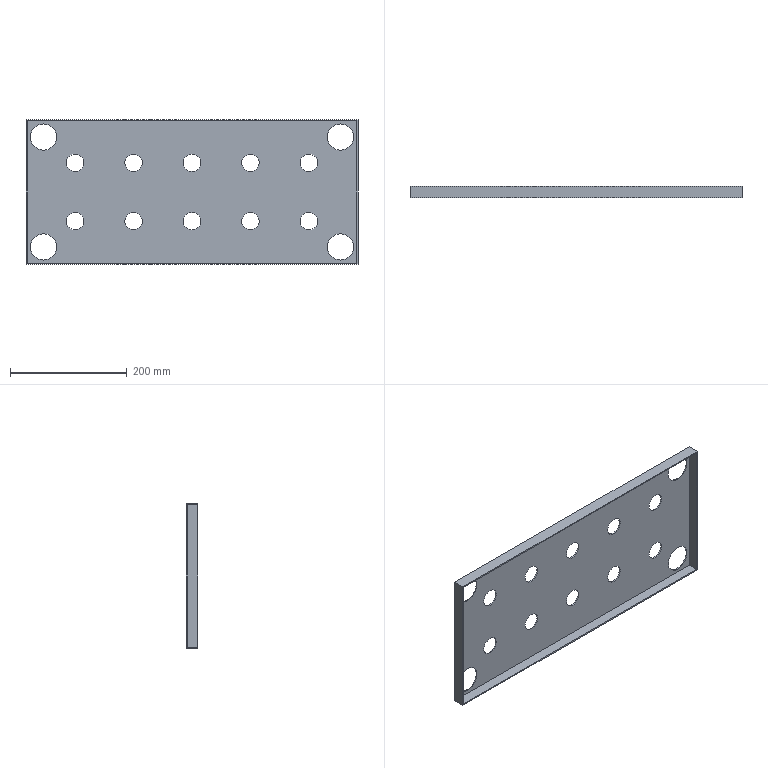Part | NX | 1 solid | 25 faces | box 568 x 20 x 248 mm | volume 313331 mm3 | cylinder 14 | plane 11 | commonest cylinder face diameters 30 x10 45 x4
STEP:
#1=CARTESIAN_POINT('',(-284.,0.,-124.));
#2=VERTEX_POINT('',#1);
#3=CARTESIAN_POINT('',(284.,0.,-124.));
#4=VERTEX_POINT('',#3);
#5=CARTESIAN_POINT('',(284.,0.,-124.));
#6=DIRECTION('',(1.,0.,0.));
#7=VECTOR('',#6,1000.);
#8=LINE('',#5,#7);
#9=EDGE_CURVE('',#2,#4,#8,.T.);
#10=ORIENTED_EDGE('',*,*,#9,.F.);
#11=CARTESIAN_POINT('',(-284.,20.,-124.));
#12=VERTEX_POINT('',#11);
#13=CARTESIAN_POINT('',(-284.,20.,-124.));
#14=DIRECTION('',(0.,-1.,0.));
#15=VECTOR('',#14,1000.);
#16=LINE('',#13,#15);
#17=EDGE_CURVE('',#12,#2,#16,.T.);
#18=ORIENTED_EDGE('',*,*,#17,.F.);
#19=CARTESIAN_POINT('',(284.,20.,-124.));
#20=VERTEX_POINT('',#19);
#21=CARTESIAN_POINT('',(284.,20.,-124.));
#22=DIRECTION('',(1.,0.,0.));
#23=VECTOR('',#22,1000.);
#24=LINE('',#21,#23);
#25=EDGE_CURVE('',#12,#20,#24,.T.);
#26=ORIENTED_EDGE('',*,*,#25,.T.);
#27=CARTESIAN_POINT('',(284.,20.,-124.));
#28=DIRECTION('',(0.,-1.,0.));
#29=VECTOR('',#28,1000.);
#30=LINE('',#27,#29);
#31=EDGE_CURVE('',#20,#4,#30,.T.);
#32=ORIENTED_EDGE('',*,*,#31,.T.);
#33=EDGE_LOOP('',(#10,#18,#26,#32));
#34=FACE_BOUND('',#33,.T.);
#35=CARTESIAN_POINT('',(284.,20.,-124.));
#36=DIRECTION('',(0.,0.,-1.));
#37=DIRECTION('',(-1.,0.,0.));
#38=AXIS2_PLACEMENT_3D('',#35,#36,#37);
#39=PLANE('',#38);
#40=ADVANCED_FACE('',(#34),#39,.T.);
#41=CARTESIAN_POINT('',(-284.,0.,124.));
#42=VERTEX_POINT('',#41);
#43=CARTESIAN_POINT('',(-284.,0.,124.));
#44=DIRECTION('',(0.,0.,-1.));
#45=VECTOR('',#44,1000.);
#46=LINE('',#43,#45);
#47=EDGE_CURVE('',#42,#2,#46,.T.);
#48=ORIENTED_EDGE('',*,*,#47,.F.);
#49=CARTESIAN_POINT('',(-284.,20.,124.));
#50=VERTEX_POINT('',#49);
#51=CARTESIAN_POINT('',(-284.,20.,124.));
#52=DIRECTION('',(0.,-1.,0.));
#53=VECTOR('',#52,1000.);
#54=LINE('',#51,#53);
#55=EDGE_CURVE('',#50,#42,#54,.T.);
#56=ORIENTED_EDGE('',*,*,#55,.F.);
#57=CARTESIAN_POINT('',(-284.,20.,124.));
#58=DIRECTION('',(0.,0.,-1.));
#59=VECTOR('',#58,1000.);
#60=LINE('',#57,#59);
#61=EDGE_CURVE('',#50,#12,#60,.T.);
#62=ORIENTED_EDGE('',*,*,#61,.T.);
#63=ORIENTED_EDGE('',*,*,#17,.T.);
#64=EDGE_LOOP('',(#48,#56,#62,#63));
#65=FACE_BOUND('',#64,.T.);
#66=CARTESIAN_POINT('',(-284.,20.,124.));
#67=DIRECTION('',(-1.,0.,0.));
#68=DIRECTION('',(0.,0.,1.));
#69=AXIS2_PLACEMENT_3D('',#66,#67,#68);
#70=PLANE('',#69);
#71=ADVANCED_FACE('',(#65),#70,.T.);
#72=CARTESIAN_POINT('',(284.,0.,124.));
#73=VERTEX_POINT('',#72);
#74=CARTESIAN_POINT('',(284.,0.,124.));
#75=DIRECTION('',(-1.,0.,0.));
#76=VECTOR('',#75,1000.);
#77=LINE('',#74,#76);
#78=EDGE_CURVE('',#73,#42,#77,.T.);
#79=ORIENTED_EDGE('',*,*,#78,.F.);
#80=CARTESIAN_POINT('',(284.,20.,124.));
#81=VERTEX_POINT('',#80);
#82=CARTESIAN_POINT('',(284.,20.,124.));
#83=DIRECTION('',(0.,-1.,0.));
#84=VECTOR('',#83,1000.);
#85=LINE('',#82,#84);
#86=EDGE_CURVE('',#81,#73,#85,.T.);
#87=ORIENTED_EDGE('',*,*,#86,.F.);
#88=CARTESIAN_POINT('',(284.,20.,124.));
#89=DIRECTION('',(-1.,0.,0.));
#90=VECTOR('',#89,1000.);
#91=LINE('',#88,#90);
#92=EDGE_CURVE('',#81,#50,#91,.T.);
#93=ORIENTED_EDGE('',*,*,#92,.T.);
#94=ORIENTED_EDGE('',*,*,#55,.T.);
#95=EDGE_LOOP('',(#79,#87,#93,#94));
#96=FACE_BOUND('',#95,.T.);
#97=CARTESIAN_POINT('',(284.,20.,124.));
#98=DIRECTION('',(0.,0.,1.));
#99=DIRECTION('',(1.,0.,0.));
#100=AXIS2_PLACEMENT_3D('',#97,#98,#99);
#101=PLANE('',#100);
#102=ADVANCED_FACE('',(#96),#101,.T.);
#103=CARTESIAN_POINT('',(284.,0.,124.));
#104=DIRECTION('',(0.,0.,1.));
#105=VECTOR('',#104,1000.);
#106=LINE('',#103,#105);
#107=EDGE_CURVE('',#4,#73,#106,.T.);
#108=ORIENTED_EDGE('',*,*,#107,.F.);
#109=ORIENTED_EDGE('',*,*,#31,.F.);
#110=CARTESIAN_POINT('',(284.,20.,124.));
#111=DIRECTION('',(0.,0.,1.));
#112=VECTOR('',#111,1000.);
#113=LINE('',#110,#112);
#114=EDGE_CURVE('',#20,#81,#113,.T.);
#115=ORIENTED_EDGE('',*,*,#114,.T.);
#116=ORIENTED_EDGE('',*,*,#86,.T.);
#117=EDGE_LOOP('',(#108,#109,#115,#116));
#118=FACE_BOUND('',#117,.T.);
#119=CARTESIAN_POINT('',(284.,20.,124.));
#120=DIRECTION('',(1.,0.,0.));
#121=DIRECTION('',(0.,0.,-1.));
#122=AXIS2_PLACEMENT_3D('',#119,#120,#121);
#123=PLANE('',#122);
#124=ADVANCED_FACE('',(#118),#123,.T.);
#125=CARTESIAN_POINT('',(-100.,20.,65.));
#126=VERTEX_POINT('',#125);
#127=CARTESIAN_POINT('',(-100.,20.,50.));
#128=DIRECTION('',(0.,1.,0.));
#129=DIRECTION('',(0.,0.,1.));
#130=AXIS2_PLACEMENT_3D('',#127,#128,#129);
#131=CIRCLE('',#130,15.);
#132=EDGE_CURVE('',#126,#126,#131,.T.);
#133=ORIENTED_EDGE('',*,*,#132,.F.);
#134=EDGE_LOOP('',(#133));
#135=FACE_BOUND('',#134,.T.);
#136=CARTESIAN_POINT('',(-200.,20.,65.));
#137=VERTEX_POINT('',#136);
#138=CARTESIAN_POINT('',(-200.,20.,50.));
#139=DIRECTION('',(0.,1.,0.));
#140=DIRECTION('',(0.,0.,1.));
#141=AXIS2_PLACEMENT_3D('',#138,#139,#140);
#142=CIRCLE('',#141,15.);
#143=EDGE_CURVE('',#137,#137,#142,.T.);
#144=ORIENTED_EDGE('',*,*,#143,.F.);
#145=EDGE_LOOP('',(#144));
#146=FACE_BOUND('',#145,.T.);
#147=CARTESIAN_POINT('',(254.,20.,116.5));
#148=VERTEX_POINT('',#147);
#149=CARTESIAN_POINT('',(254.,20.,94.));
#150=DIRECTION('',(0.,1.,0.));
#151=DIRECTION('',(0.,0.,1.));
#152=AXIS2_PLACEMENT_3D('',#149,#150,#151);
#153=CIRCLE('',#152,22.5);
#154=EDGE_CURVE('',#148,#148,#153,.T.);
#155=ORIENTED_EDGE('',*,*,#154,.F.);
#156=EDGE_LOOP('',(#155));
#157=FACE_BOUND('',#156,.T.);
#158=CARTESIAN_POINT('',(254.,20.,-71.5));
#159=VERTEX_POINT('',#158);
#160=CARTESIAN_POINT('',(254.,20.,-94.));
#161=DIRECTION('',(0.,1.,0.));
#162=DIRECTION('',(0.,0.,1.));
#163=AXIS2_PLACEMENT_3D('',#160,#161,#162);
#164=CIRCLE('',#163,22.5);
#165=EDGE_CURVE('',#159,#159,#164,.T.);
#166=ORIENTED_EDGE('',*,*,#165,.F.);
#167=EDGE_LOOP('',(#166));
#168=FACE_BOUND('',#167,.T.);
#169=CARTESIAN_POINT('',(-254.,20.,116.5));
#170=VERTEX_POINT('',#169);
#171=CARTESIAN_POINT('',(-254.,20.,94.));
#172=DIRECTION('',(0.,1.,0.));
#173=DIRECTION('',(0.,0.,1.));
#174=AXIS2_PLACEMENT_3D('',#171,#172,#173);
#175=CIRCLE('',#174,22.5);
#176=EDGE_CURVE('',#170,#170,#175,.T.);
#177=ORIENTED_EDGE('',*,*,#176,.F.);
#178=EDGE_LOOP('',(#177));
#179=FACE_BOUND('',#178,.T.);
#180=CARTESIAN_POINT('',(-254.,20.,-71.5));
#181=VERTEX_POINT('',#180);
#182=CARTESIAN_POINT('',(-254.,20.,-94.));
#183=DIRECTION('',(0.,1.,0.));
#184=DIRECTION('',(0.,0.,1.));
#185=AXIS2_PLACEMENT_3D('',#182,#183,#184);
#186=CIRCLE('',#185,22.5);
#187=EDGE_CURVE('',#181,#181,#186,.T.);
#188=ORIENTED_EDGE('',*,*,#187,.F.);
#189=EDGE_LOOP('',(#188));
#190=FACE_BOUND('',#189,.T.);
#191=ORIENTED_EDGE('',*,*,#25,.F.);
#192=ORIENTED_EDGE('',*,*,#61,.F.);
#193=ORIENTED_EDGE('',*,*,#92,.F.);
#194=ORIENTED_EDGE('',*,*,#114,.F.);
#195=EDGE_LOOP('',(#191,#192,#193,#194));
#196=FACE_BOUND('',#195,.T.);
#197=CARTESIAN_POINT('',(0.,20.,65.));
#198=VERTEX_POINT('',#197);
#199=CARTESIAN_POINT('',(0.,20.,50.));
#200=DIRECTION('',(0.,1.,0.));
#201=DIRECTION('',(0.,0.,1.));
#202=AXIS2_PLACEMENT_3D('',#199,#200,#201);
#203=CIRCLE('',#202,15.);
#204=EDGE_CURVE('',#198,#198,#203,.T.);
#205=ORIENTED_EDGE('',*,*,#204,.F.);
#206=EDGE_LOOP('',(#205));
#207=FACE_BOUND('',#206,.T.);
#208=CARTESIAN_POINT('',(100.,20.,65.));
#209=VERTEX_POINT('',#208);
#210=CARTESIAN_POINT('',(100.,20.,50.));
#211=DIRECTION('',(0.,1.,0.));
#212=DIRECTION('',(0.,0.,1.));
#213=AXIS2_PLACEMENT_3D('',#210,#211,#212);
#214=CIRCLE('',#213,15.);
#215=EDGE_CURVE('',#209,#209,#214,.T.);
#216=ORIENTED_EDGE('',*,*,#215,.F.);
#217=EDGE_LOOP('',(#216));
#218=FACE_BOUND('',#217,.T.);
#219=CARTESIAN_POINT('',(200.,20.,65.));
#220=VERTEX_POINT('',#219);
#221=CARTESIAN_POINT('',(200.,20.,50.));
#222=DIRECTION('',(0.,1.,0.));
#223=DIRECTION('',(0.,0.,1.));
#224=AXIS2_PLACEMENT_3D('',#221,#222,#223);
#225=CIRCLE('',#224,15.);
#226=EDGE_CURVE('',#220,#220,#225,.T.);
#227=ORIENTED_EDGE('',*,*,#226,.F.);
#228=EDGE_LOOP('',(#227));
#229=FACE_BOUND('',#228,.T.);
#230=CARTESIAN_POINT('',(-200.,20.,-35.));
#231=VERTEX_POINT('',#230);
#232=CARTESIAN_POINT('',(-200.,20.,-50.));
#233=DIRECTION('',(0.,1.,0.));
#234=DIRECTION('',(0.,0.,1.));
#235=AXIS2_PLACEMENT_3D('',#232,#233,#234);
#236=CIRCLE('',#235,15.);
#237=EDGE_CURVE('',#231,#231,#236,.T.);
#238=ORIENTED_EDGE('',*,*,#237,.F.);
#239=EDGE_LOOP('',(#238));
#240=FACE_BOUND('',#239,.T.);
#241=CARTESIAN_POINT('',(-100.,20.,-35.));
#242=VERTEX_POINT('',#241);
#243=CARTESIAN_POINT('',(-100.,20.,-50.));
#244=DIRECTION('',(0.,1.,0.));
#245=DIRECTION('',(0.,0.,1.));
#246=AXIS2_PLACEMENT_3D('',#243,#244,#245);
#247=CIRCLE('',#246,15.);
#248=EDGE_CURVE('',#242,#242,#247,.T.);
#249=ORIENTED_EDGE('',*,*,#248,.F.);
#250=EDGE_LOOP('',(#249));
#251=FACE_BOUND('',#250,.T.);
#252=CARTESIAN_POINT('',(0.,20.,-35.));
#253=VERTEX_POINT('',#252);
#254=CARTESIAN_POINT('',(0.,20.,-50.));
#255=DIRECTION('',(0.,1.,0.));
#256=DIRECTION('',(0.,0.,1.));
#257=AXIS2_PLACEMENT_3D('',#254,#255,#256);
#258=CIRCLE('',#257,15.);
#259=EDGE_CURVE('',#253,#253,#258,.T.);
#260=ORIENTED_EDGE('',*,*,#259,.F.);
#261=EDGE_LOOP('',(#260));
#262=FACE_BOUND('',#261,.T.);
#263=CARTESIAN_POINT('',(100.,20.,-35.));
#264=VERTEX_POINT('',#263);
#265=CARTESIAN_POINT('',(100.,20.,-50.));
#266=DIRECTION('',(0.,1.,0.));
#267=DIRECTION('',(0.,0.,1.));
#268=AXIS2_PLACEMENT_3D('',#265,#266,#267);
#269=CIRCLE('',#268,15.);
#270=EDGE_CURVE('',#264,#264,#269,.T.);
#271=ORIENTED_EDGE('',*,*,#270,.F.);
#272=EDGE_LOOP('',(#271));
#273=FACE_BOUND('',#272,.T.);
#274=CARTESIAN_POINT('',(200.,20.,-35.));
#275=VERTEX_POINT('',#274);
#276=CARTESIAN_POINT('',(200.,20.,-50.));
#277=DIRECTION('',(0.,1.,0.));
#278=DIRECTION('',(0.,0.,1.));
#279=AXIS2_PLACEMENT_3D('',#276,#277,#278);
#280=CIRCLE('',#279,15.);
#281=EDGE_CURVE('',#275,#275,#280,.T.);
#282=ORIENTED_EDGE('',*,*,#281,.F.);
#283=EDGE_LOOP('',(#282));
#284=FACE_BOUND('',#283,.T.);
#285=CARTESIAN_POINT('',(0.,20.,0.));
#286=DIRECTION('',(0.,-1.,0.));
#287=DIRECTION('',(0.,0.,-1.));
#288=AXIS2_PLACEMENT_3D('',#285,#286,#287);
#289=PLANE('',#288);
#290=ADVANCED_FACE('',(#135,#146,#157,#168,#179,#190,#196,#207,#218,#229,#240,#251,#262,#273,#284),#289,.F.);
#291=CARTESIAN_POINT('',(-282.,0.,-122.));
#292=VERTEX_POINT('',#291);
#293=CARTESIAN_POINT('',(282.,0.,-122.));
#294=VERTEX_POINT('',#293);
#295=CARTESIAN_POINT('',(0.,0.,-122.));
#296=DIRECTION('',(1.,0.,0.));
#297=VECTOR('',#296,1000.);
#298=LINE('',#295,#297);
#299=EDGE_CURVE('',#292,#294,#298,.T.);
#300=ORIENTED_EDGE('',*,*,#299,.F.);
#301=CARTESIAN_POINT('',(-282.,0.,122.));
#302=VERTEX_POINT('',#301);
#303=CARTESIAN_POINT('',(-282.,0.,0.));
#304=DIRECTION('',(0.,0.,-1.));
#305=VECTOR('',#304,1000.);
#306=LINE('',#303,#305);
#307=EDGE_CURVE('',#302,#292,#306,.T.);
#308=ORIENTED_EDGE('',*,*,#307,.F.);
#309=CARTESIAN_POINT('',(282.,0.,122.));
#310=VERTEX_POINT('',#309);
#311=CARTESIAN_POINT('',(0.,0.,122.));
#312=DIRECTION('',(-1.,0.,0.));
#313=VECTOR('',#312,1000.);
#314=LINE('',#311,#313);
#315=EDGE_CURVE('',#310,#302,#314,.T.);
#316=ORIENTED_EDGE('',*,*,#315,.F.);
#317=CARTESIAN_POINT('',(282.,0.,0.));
#318=DIRECTION('',(0.,0.,1.));
#319=VECTOR('',#318,1000.);
#320=LINE('',#317,#319);
#321=EDGE_CURVE('',#294,#310,#320,.T.);
#322=ORIENTED_EDGE('',*,*,#321,.F.);
#323=EDGE_LOOP('',(#300,#308,#316,#322));
#324=FACE_BOUND('',#323,.T.);
#325=ORIENTED_EDGE('',*,*,#9,.T.);
#326=ORIENTED_EDGE('',*,*,#107,.T.);
#327=ORIENTED_EDGE('',*,*,#78,.T.);
#328=ORIENTED_EDGE('',*,*,#47,.T.);
#329=EDGE_LOOP('',(#325,#326,#327,#328));
#330=FACE_BOUND('',#329,.T.);
#331=CARTESIAN_POINT('',(0.,0.,0.));
#332=DIRECTION('',(0.,-1.,0.));
#333=DIRECTION('',(0.,0.,-1.));
#334=AXIS2_PLACEMENT_3D('',#331,#332,#333);
#335=PLANE('',#334);
#336=ADVANCED_FACE('',(#324,#330),#335,.T.);
#337=ORIENTED_EDGE('',*,*,#299,.T.);
#338=CARTESIAN_POINT('',(282.,18.,-122.));
#339=VERTEX_POINT('',#338);
#340=CARTESIAN_POINT('',(282.,20.,-122.));
#341=DIRECTION('',(0.,-1.,0.));
#342=VECTOR('',#341,1000.);
#343=LINE('',#340,#342);
#344=EDGE_CURVE('',#339,#294,#343,.T.);
#345=ORIENTED_EDGE('',*,*,#344,.F.);
#346=CARTESIAN_POINT('',(-282.,18.,-122.));
#347=VERTEX_POINT('',#346);
#348=CARTESIAN_POINT('',(0.,18.,-122.));
#349=DIRECTION('',(1.,0.,0.));
#350=VECTOR('',#349,1000.);
#351=LINE('',#348,#350);
#352=EDGE_CURVE('',#347,#339,#351,.T.);
#353=ORIENTED_EDGE('',*,*,#352,.F.);
#354=CARTESIAN_POINT('',(-282.,20.,-122.));
#355=DIRECTION('',(0.,-1.,0.));
#356=VECTOR('',#355,1000.);
#357=LINE('',#354,#356);
#358=EDGE_CURVE('',#347,#292,#357,.T.);
#359=ORIENTED_EDGE('',*,*,#358,.T.);
#360=EDGE_LOOP('',(#337,#345,#353,#359));
#361=FACE_BOUND('',#360,.T.);
#362=CARTESIAN_POINT('',(284.,20.,-122.));
#363=DIRECTION('',(0.,0.,-1.));
#364=DIRECTION('',(-1.,0.,0.));
#365=AXIS2_PLACEMENT_3D('',#362,#363,#364);
#366=PLANE('',#365);
#367=ADVANCED_FACE('',(#361),#366,.F.);
#368=ORIENTED_EDGE('',*,*,#307,.T.);
#369=ORIENTED_EDGE('',*,*,#358,.F.);
#370=CARTESIAN_POINT('',(-282.,18.,122.));
#371=VERTEX_POINT('',#370);
#372=CARTESIAN_POINT('',(-282.,18.,0.));
#373=DIRECTION('',(0.,0.,-1.));
#374=VECTOR('',#373,1000.);
#375=LINE('',#372,#374);
#376=EDGE_CURVE('',#371,#347,#375,.T.);
#377=ORIENTED_EDGE('',*,*,#376,.F.);
#378=CARTESIAN_POINT('',(-282.,20.,122.));
#379=DIRECTION('',(0.,-1.,0.));
#380=VECTOR('',#379,1000.);
#381=LINE('',#378,#380);
#382=EDGE_CURVE('',#371,#302,#381,.T.);
#383=ORIENTED_EDGE('',*,*,#382,.T.);
#384=EDGE_LOOP('',(#368,#369,#377,#383));
#385=FACE_BOUND('',#384,.T.);
#386=CARTESIAN_POINT('',(-282.,20.,124.));
#387=DIRECTION('',(-1.,0.,0.));
#388=DIRECTION('',(0.,0.,1.));
#389=AXIS2_PLACEMENT_3D('',#386,#387,#388);
#390=PLANE('',#389);
#391=ADVANCED_FACE('',(#385),#390,.F.);
#392=ORIENTED_EDGE('',*,*,#315,.T.);
#393=ORIENTED_EDGE('',*,*,#382,.F.);
#394=CARTESIAN_POINT('',(282.,18.,122.));
#395=VERTEX_POINT('',#394);
#396=CARTESIAN_POINT('',(0.,18.,122.));
#397=DIRECTION('',(-1.,0.,0.));
#398=VECTOR('',#397,1000.);
#399=LINE('',#396,#398);
#400=EDGE_CURVE('',#395,#371,#399,.T.);
#401=ORIENTED_EDGE('',*,*,#400,.F.);
#402=CARTESIAN_POINT('',(282.,20.,122.));
#403=DIRECTION('',(0.,-1.,0.));
#404=VECTOR('',#403,1000.);
#405=LINE('',#402,#404);
#406=EDGE_CURVE('',#395,#310,#405,.T.);
#407=ORIENTED_EDGE('',*,*,#406,.T.);
#408=EDGE_LOOP('',(#392,#393,#401,#407));
#409=FACE_BOUND('',#408,.T.);
#410=CARTESIAN_POINT('',(284.,20.,122.));
#411=DIRECTION('',(0.,0.,1.));
#412=DIRECTION('',(1.,0.,0.));
#413=AXIS2_PLACEMENT_3D('',#410,#411,#412);
#414=PLANE('',#413);
#415=ADVANCED_FACE('',(#409),#414,.F.);
#416=ORIENTED_EDGE('',*,*,#321,.T.);
#417=ORIENTED_EDGE('',*,*,#406,.F.);
#418=CARTESIAN_POINT('',(282.,18.,0.));
#419=DIRECTION('',(0.,0.,1.));
#420=VECTOR('',#419,1000.);
#421=LINE('',#418,#420);
#422=EDGE_CURVE('',#339,#395,#421,.T.);
#423=ORIENTED_EDGE('',*,*,#422,.F.);
#424=ORIENTED_EDGE('',*,*,#344,.T.);
#425=EDGE_LOOP('',(#416,#417,#423,#424));
#426=FACE_BOUND('',#425,.T.);
#427=CARTESIAN_POINT('',(282.,20.,124.));
#428=DIRECTION('',(1.,0.,0.));
#429=DIRECTION('',(0.,0.,-1.));
#430=AXIS2_PLACEMENT_3D('',#427,#428,#429);
#431=PLANE('',#430);
#432=ADVANCED_FACE('',(#426),#431,.F.);
#433=CARTESIAN_POINT('',(-100.,18.,35.));
#434=VERTEX_POINT('',#433);
#435=CARTESIAN_POINT('',(-100.,18.,50.));
#436=DIRECTION('',(0.,-1.,0.));
#437=DIRECTION('',(0.,0.,-1.));
#438=AXIS2_PLACEMENT_3D('',#435,#436,#437);
#439=CIRCLE('',#438,15.);
#440=EDGE_CURVE('',#434,#434,#439,.T.);
#441=ORIENTED_EDGE('',*,*,#440,.F.);
#442=EDGE_LOOP('',(#441));
#443=FACE_BOUND('',#442,.T.);
#444=CARTESIAN_POINT('',(-200.,18.,35.));
#445=VERTEX_POINT('',#444);
#446=CARTESIAN_POINT('',(-200.,18.,50.));
#447=DIRECTION('',(0.,-1.,0.));
#448=DIRECTION('',(0.,0.,-1.));
#449=AXIS2_PLACEMENT_3D('',#446,#447,#448);
#450=CIRCLE('',#449,15.);
#451=EDGE_CURVE('',#445,#445,#450,.T.);
#452=ORIENTED_EDGE('',*,*,#451,.F.);
#453=EDGE_LOOP('',(#452));
#454=FACE_BOUND('',#453,.T.);
#455=CARTESIAN_POINT('',(254.,18.,71.5));
#456=VERTEX_POINT('',#455);
#457=CARTESIAN_POINT('',(254.,18.,94.));
#458=DIRECTION('',(0.,-1.,0.));
#459=DIRECTION('',(0.,0.,-1.));
#460=AXIS2_PLACEMENT_3D('',#457,#458,#459);
#461=CIRCLE('',#460,22.5);
#462=EDGE_CURVE('',#456,#456,#461,.T.);
#463=ORIENTED_EDGE('',*,*,#462,.F.);
#464=EDGE_LOOP('',(#463));
#465=FACE_BOUND('',#464,.T.);
#466=CARTESIAN_POINT('',(254.,18.,-116.5));
#467=VERTEX_POINT('',#466);
#468=CARTESIAN_POINT('',(254.,18.,-94.));
#469=DIRECTION('',(0.,-1.,0.));
#470=DIRECTION('',(0.,0.,-1.));
#471=AXIS2_PLACEMENT_3D('',#468,#469,#470);
#472=CIRCLE('',#471,22.5);
#473=EDGE_CURVE('',#467,#467,#472,.T.);
#474=ORIENTED_EDGE('',*,*,#473,.F.);
#475=EDGE_LOOP('',(#474));
#476=FACE_BOUND('',#475,.T.);
#477=CARTESIAN_POINT('',(-254.,18.,71.5));
#478=VERTEX_POINT('',#477);
#479=CARTESIAN_POINT('',(-254.,18.,94.));
#480=DIRECTION('',(0.,-1.,0.));
#481=DIRECTION('',(0.,0.,-1.));
#482=AXIS2_PLACEMENT_3D('',#479,#480,#481);
#483=CIRCLE('',#482,22.5);
#484=EDGE_CURVE('',#478,#478,#483,.T.);
#485=ORIENTED_EDGE('',*,*,#484,.F.);
#486=EDGE_LOOP('',(#485));
#487=FACE_BOUND('',#486,.T.);
#488=CARTESIAN_POINT('',(-254.,18.,-116.5));
#489=VERTEX_POINT('',#488);
#490=CARTESIAN_POINT('',(-254.,18.,-94.));
#491=DIRECTION('',(0.,-1.,0.));
#492=DIRECTION('',(0.,0.,-1.));
#493=AXIS2_PLACEMENT_3D('',#490,#491,#492);
#494=CIRCLE('',#493,22.5);
#495=EDGE_CURVE('',#489,#489,#494,.T.);
#496=ORIENTED_EDGE('',*,*,#495,.F.);
#497=EDGE_LOOP('',(#496));
#498=FACE_BOUND('',#497,.T.);
#499=ORIENTED_EDGE('',*,*,#352,.T.);
#500=ORIENTED_EDGE('',*,*,#422,.T.);
#501=ORIENTED_EDGE('',*,*,#400,.T.);
#502=ORIENTED_EDGE('',*,*,#376,.T.);
#503=EDGE_LOOP('',(#499,#500,#501,#502));
#504=FACE_BOUND('',#503,.T.);
#505=CARTESIAN_POINT('',(0.,18.,35.));
#506=VERTEX_POINT('',#505);
#507=CARTESIAN_POINT('',(0.,18.,50.));
#508=DIRECTION('',(0.,-1.,0.));
#509=DIRECTION('',(0.,0.,-1.));
#510=AXIS2_PLACEMENT_3D('',#507,#508,#509);
#511=CIRCLE('',#510,15.);
#512=EDGE_CURVE('',#506,#506,#511,.T.);
#513=ORIENTED_EDGE('',*,*,#512,.F.);
#514=EDGE_LOOP('',(#513));
#515=FACE_BOUND('',#514,.T.);
#516=CARTESIAN_POINT('',(100.,18.,35.));
#517=VERTEX_POINT('',#516);
#518=CARTESIAN_POINT('',(100.,18.,50.));
#519=DIRECTION('',(0.,-1.,0.));
#520=DIRECTION('',(0.,0.,-1.));
#521=AXIS2_PLACEMENT_3D('',#518,#519,#520);
#522=CIRCLE('',#521,15.);
#523=EDGE_CURVE('',#517,#517,#522,.T.);
#524=ORIENTED_EDGE('',*,*,#523,.F.);
#525=EDGE_LOOP('',(#524));
#526=FACE_BOUND('',#525,.T.);
#527=CARTESIAN_POINT('',(200.,18.,35.));
#528=VERTEX_POINT('',#527);
#529=CARTESIAN_POINT('',(200.,18.,50.));
#530=DIRECTION('',(0.,-1.,0.));
#531=DIRECTION('',(0.,0.,-1.));
#532=AXIS2_PLACEMENT_3D('',#529,#530,#531);
#533=CIRCLE('',#532,15.);
#534=EDGE_CURVE('',#528,#528,#533,.T.);
#535=ORIENTED_EDGE('',*,*,#534,.F.);
#536=EDGE_LOOP('',(#535));
#537=FACE_BOUND('',#536,.T.);
#538=CARTESIAN_POINT('',(-200.,18.,-65.));
#539=VERTEX_POINT('',#538);
#540=CARTESIAN_POINT('',(-200.,18.,-50.));
#541=DIRECTION('',(0.,-1.,0.));
#542=DIRECTION('',(0.,0.,-1.));
#543=AXIS2_PLACEMENT_3D('',#540,#541,#542);
#544=CIRCLE('',#543,15.);
#545=EDGE_CURVE('',#539,#539,#544,.T.);
#546=ORIENTED_EDGE('',*,*,#545,.F.);
#547=EDGE_LOOP('',(#546));
#548=FACE_BOUND('',#547,.T.);
#549=CARTESIAN_POINT('',(-100.,18.,-65.));
#550=VERTEX_POINT('',#549);
#551=CARTESIAN_POINT('',(-100.,18.,-50.));
#552=DIRECTION('',(0.,-1.,0.));
#553=DIRECTION('',(0.,0.,-1.));
#554=AXIS2_PLACEMENT_3D('',#551,#552,#553);
#555=CIRCLE('',#554,15.);
#556=EDGE_CURVE('',#550,#550,#555,.T.);
#557=ORIENTED_EDGE('',*,*,#556,.F.);
#558=EDGE_LOOP('',(#557));
#559=FACE_BOUND('',#558,.T.);
#560=CARTESIAN_POINT('',(0.,18.,-65.));
#561=VERTEX_POINT('',#560);
#562=CARTESIAN_POINT('',(0.,18.,-50.));
#563=DIRECTION('',(0.,-1.,0.));
#564=DIRECTION('',(0.,0.,-1.));
#565=AXIS2_PLACEMENT_3D('',#562,#563,#564);
#566=CIRCLE('',#565,15.);
#567=EDGE_CURVE('',#561,#561,#566,.T.);
#568=ORIENTED_EDGE('',*,*,#567,.F.);
#569=EDGE_LOOP('',(#568));
#570=FACE_BOUND('',#569,.T.);
#571=CARTESIAN_POINT('',(100.,18.,-65.));
#572=VERTEX_POINT('',#571);
#573=CARTESIAN_POINT('',(100.,18.,-50.));
#574=DIRECTION('',(0.,-1.,0.));
#575=DIRECTION('',(0.,0.,-1.));
#576=AXIS2_PLACEMENT_3D('',#573,#574,#575);
#577=CIRCLE('',#576,15.);
#578=EDGE_CURVE('',#572,#572,#577,.T.);
#579=ORIENTED_EDGE('',*,*,#578,.F.);
#580=EDGE_LOOP('',(#579));
#581=FACE_BOUND('',#580,.T.);
#582=CARTESIAN_POINT('',(200.,18.,-65.));
#583=VERTEX_POINT('',#582);
#584=CARTESIAN_POINT('',(200.,18.,-50.));
#585=DIRECTION('',(0.,-1.,0.));
#586=DIRECTION('',(0.,0.,-1.));
#587=AXIS2_PLACEMENT_3D('',#584,#585,#586);
#588=CIRCLE('',#587,15.);
#589=EDGE_CURVE('',#583,#583,#588,.T.);
#590=ORIENTED_EDGE('',*,*,#589,.F.);
#591=EDGE_LOOP('',(#590));
#592=FACE_BOUND('',#591,.T.);
#593=CARTESIAN_POINT('',(0.,18.,0.));
#594=DIRECTION('',(0.,-1.,0.));
#595=DIRECTION('',(0.,0.,-1.));
#596=AXIS2_PLACEMENT_3D('',#593,#594,#595);
#597=PLANE('',#596);
#598=ADVANCED_FACE('',(#443,#454,#465,#476,#487,#498,#504,#515,#526,#537,#548,#559,#570,#581,#592),#597,.T.);
#599=ORIENTED_EDGE('',*,*,#495,.T.);
#600=EDGE_LOOP('',(#599));
#601=FACE_BOUND('',#600,.T.);
#602=ORIENTED_EDGE('',*,*,#187,.T.);
#603=EDGE_LOOP('',(#602));
#604=FACE_BOUND('',#603,.T.);
#605=CARTESIAN_POINT('',(-254.,0.,-94.));
#606=DIRECTION('',(0.,1.,0.));
#607=DIRECTION('',(0.,0.,1.));
#608=AXIS2_PLACEMENT_3D('',#605,#606,#607);
#609=CYLINDRICAL_SURFACE('',#608,22.5);
#610=ADVANCED_FACE('',(#601,#604),#609,.F.);
#611=ORIENTED_EDGE('',*,*,#484,.T.);
#612=EDGE_LOOP('',(#611));
#613=FACE_BOUND('',#612,.T.);
#614=ORIENTED_EDGE('',*,*,#176,.T.);
#615=EDGE_LOOP('',(#614));
#616=FACE_BOUND('',#615,.T.);
#617=CARTESIAN_POINT('',(-254.,0.,94.));
#618=DIRECTION('',(0.,1.,0.));
#619=DIRECTION('',(0.,0.,1.));
#620=AXIS2_PLACEMENT_3D('',#617,#618,#619);
#621=CYLINDRICAL_SURFACE('',#620,22.5);
#622=ADVANCED_FACE('',(#613,#616),#621,.F.);
#623=ORIENTED_EDGE('',*,*,#473,.T.);
#624=EDGE_LOOP('',(#623));
#625=FACE_BOUND('',#624,.T.);
#626=ORIENTED_EDGE('',*,*,#165,.T.);
#627=EDGE_LOOP('',(#626));
#628=FACE_BOUND('',#627,.T.);
#629=CARTESIAN_POINT('',(254.,0.,-94.));
#630=DIRECTION('',(0.,1.,0.));
#631=DIRECTION('',(0.,0.,1.));
#632=AXIS2_PLACEMENT_3D('',#629,#630,#631);
#633=CYLINDRICAL_SURFACE('',#632,22.5);
#634=ADVANCED_FACE('',(#625,#628),#633,.F.);
#635=ORIENTED_EDGE('',*,*,#462,.T.);
#636=EDGE_LOOP('',(#635));
#637=FACE_BOUND('',#636,.T.);
#638=ORIENTED_EDGE('',*,*,#154,.T.);
#639=EDGE_LOOP('',(#638));
#640=FACE_BOUND('',#639,.T.);
#641=CARTESIAN_POINT('',(254.,0.,94.));
#642=DIRECTION('',(0.,1.,0.));
#643=DIRECTION('',(0.,0.,1.));
#644=AXIS2_PLACEMENT_3D('',#641,#642,#643);
#645=CYLINDRICAL_SURFACE('',#644,22.5);
#646=ADVANCED_FACE('',(#637,#640),#645,.F.);
#647=ORIENTED_EDGE('',*,*,#451,.T.);
#648=EDGE_LOOP('',(#647));
#649=FACE_BOUND('',#648,.T.);
#650=ORIENTED_EDGE('',*,*,#143,.T.);
#651=EDGE_LOOP('',(#650));
#652=FACE_BOUND('',#651,.T.);
#653=CARTESIAN_POINT('',(-200.,0.,50.));
#654=DIRECTION('',(0.,1.,0.));
#655=DIRECTION('',(0.,0.,1.));
#656=AXIS2_PLACEMENT_3D('',#653,#654,#655);
#657=CYLINDRICAL_SURFACE('',#656,15.);
#658=ADVANCED_FACE('',(#649,#652),#657,.F.);
#659=ORIENTED_EDGE('',*,*,#440,.T.);
#660=EDGE_LOOP('',(#659));
#661=FACE_BOUND('',#660,.T.);
#662=ORIENTED_EDGE('',*,*,#132,.T.);
#663=EDGE_LOOP('',(#662));
#664=FACE_BOUND('',#663,.T.);
#665=CARTESIAN_POINT('',(-100.,0.,50.));
#666=DIRECTION('',(0.,1.,0.));
#667=DIRECTION('',(0.,0.,1.));
#668=AXIS2_PLACEMENT_3D('',#665,#666,#667);
#669=CYLINDRICAL_SURFACE('',#668,15.);
#670=ADVANCED_FACE('',(#661,#664),#669,.F.);
#671=ORIENTED_EDGE('',*,*,#512,.T.);
#672=EDGE_LOOP('',(#671));
#673=FACE_BOUND('',#672,.T.);
#674=ORIENTED_EDGE('',*,*,#204,.T.);
#675=EDGE_LOOP('',(#674));
#676=FACE_BOUND('',#675,.T.);
#677=CARTESIAN_POINT('',(0.,0.,50.));
#678=DIRECTION('',(0.,1.,0.));
#679=DIRECTION('',(0.,0.,1.));
#680=AXIS2_PLACEMENT_3D('',#677,#678,#679);
#681=CYLINDRICAL_SURFACE('',#680,15.);
#682=ADVANCED_FACE('',(#673,#676),#681,.F.);
#683=ORIENTED_EDGE('',*,*,#523,.T.);
#684=EDGE_LOOP('',(#683));
#685=FACE_BOUND('',#684,.T.);
#686=ORIENTED_EDGE('',*,*,#215,.T.);
#687=EDGE_LOOP('',(#686));
#688=FACE_BOUND('',#687,.T.);
#689=CARTESIAN_POINT('',(100.,0.,50.));
#690=DIRECTION('',(0.,1.,0.));
#691=DIRECTION('',(0.,0.,1.));
#692=AXIS2_PLACEMENT_3D('',#689,#690,#691);
#693=CYLINDRICAL_SURFACE('',#692,15.);
#694=ADVANCED_FACE('',(#685,#688),#693,.F.);
#695=ORIENTED_EDGE('',*,*,#534,.T.);
#696=EDGE_LOOP('',(#695));
#697=FACE_BOUND('',#696,.T.);
#698=ORIENTED_EDGE('',*,*,#226,.T.);
#699=EDGE_LOOP('',(#698));
#700=FACE_BOUND('',#699,.T.);
#701=CARTESIAN_POINT('',(200.,0.,50.));
#702=DIRECTION('',(0.,1.,0.));
#703=DIRECTION('',(0.,0.,1.));
#704=AXIS2_PLACEMENT_3D('',#701,#702,#703);
#705=CYLINDRICAL_SURFACE('',#704,15.);
#706=ADVANCED_FACE('',(#697,#700),#705,.F.);
#707=ORIENTED_EDGE('',*,*,#545,.T.);
#708=EDGE_LOOP('',(#707));
#709=FACE_BOUND('',#708,.T.);
#710=ORIENTED_EDGE('',*,*,#237,.T.);
#711=EDGE_LOOP('',(#710));
#712=FACE_BOUND('',#711,.T.);
#713=CARTESIAN_POINT('',(-200.,0.,-50.));
#714=DIRECTION('',(0.,1.,0.));
#715=DIRECTION('',(0.,0.,1.));
#716=AXIS2_PLACEMENT_3D('',#713,#714,#715);
#717=CYLINDRICAL_SURFACE('',#716,15.);
#718=ADVANCED_FACE('',(#709,#712),#717,.F.);
#719=ORIENTED_EDGE('',*,*,#556,.T.);
#720=EDGE_LOOP('',(#719));
#721=FACE_BOUND('',#720,.T.);
#722=ORIENTED_EDGE('',*,*,#248,.T.);
#723=EDGE_LOOP('',(#722));
#724=FACE_BOUND('',#723,.T.);
#725=CARTESIAN_POINT('',(-100.,0.,-50.));
#726=DIRECTION('',(0.,1.,0.));
#727=DIRECTION('',(0.,0.,1.));
#728=AXIS2_PLACEMENT_3D('',#725,#726,#727);
#729=CYLINDRICAL_SURFACE('',#728,15.);
#730=ADVANCED_FACE('',(#721,#724),#729,.F.);
#731=ORIENTED_EDGE('',*,*,#567,.T.);
#732=EDGE_LOOP('',(#731));
#733=FACE_BOUND('',#732,.T.);
#734=ORIENTED_EDGE('',*,*,#259,.T.);
#735=EDGE_LOOP('',(#734));
#736=FACE_BOUND('',#735,.T.);
#737=CARTESIAN_POINT('',(0.,0.,-50.));
#738=DIRECTION('',(0.,1.,0.));
#739=DIRECTION('',(0.,0.,1.));
#740=AXIS2_PLACEMENT_3D('',#737,#738,#739);
#741=CYLINDRICAL_SURFACE('',#740,15.);
#742=ADVANCED_FACE('',(#733,#736),#741,.F.);
#743=ORIENTED_EDGE('',*,*,#578,.T.);
#744=EDGE_LOOP('',(#743));
#745=FACE_BOUND('',#744,.T.);
#746=ORIENTED_EDGE('',*,*,#270,.T.);
#747=EDGE_LOOP('',(#746));
#748=FACE_BOUND('',#747,.T.);
#749=CARTESIAN_POINT('',(100.,0.,-50.));
#750=DIRECTION('',(0.,1.,0.));
#751=DIRECTION('',(0.,0.,1.));
#752=AXIS2_PLACEMENT_3D('',#749,#750,#751);
#753=CYLINDRICAL_SURFACE('',#752,15.);
#754=ADVANCED_FACE('',(#745,#748),#753,.F.);
#755=ORIENTED_EDGE('',*,*,#589,.T.);
#756=EDGE_LOOP('',(#755));
#757=FACE_BOUND('',#756,.T.);
#758=ORIENTED_EDGE('',*,*,#281,.T.);
#759=EDGE_LOOP('',(#758));
#760=FACE_BOUND('',#759,.T.);
#761=CARTESIAN_POINT('',(200.,0.,-50.));
#762=DIRECTION('',(0.,1.,0.));
#763=DIRECTION('',(0.,0.,1.));
#764=AXIS2_PLACEMENT_3D('',#761,#762,#763);
#765=CYLINDRICAL_SURFACE('',#764,15.);
#766=ADVANCED_FACE('',(#757,#760),#765,.F.);
#767=CLOSED_SHELL('',(#40,#71,#102,#124,#290,#336,#367,#391,#415,#432,#598,#610,#622,#634,#646,#658,#670,#682,#694,#706,#718,#730,#742,#754,#766));
#768=MANIFOLD_SOLID_BREP('',#767);
#769=(LENGTH_UNIT()NAMED_UNIT(*)SI_UNIT(.MILLI.,.METRE.));
#770=UNCERTAINTY_MEASURE_WITH_UNIT(LENGTH_MEASURE(0.00001),#769,'','');
#771=(NAMED_UNIT(*)PLANE_ANGLE_UNIT()SI_UNIT($,.RADIAN.));
#772=(NAMED_UNIT(*)SI_UNIT($,.STERADIAN.)SOLID_ANGLE_UNIT());
#773=(GEOMETRIC_REPRESENTATION_CONTEXT(3)GLOBAL_UNCERTAINTY_ASSIGNED_CONTEXT((#770))GLOBAL_UNIT_ASSIGNED_CONTEXT((#769,#771,#772))REPRESENTATION_CONTEXT('',''));
#774=ADVANCED_BREP_SHAPE_REPRESENTATION('',(#768),#773);